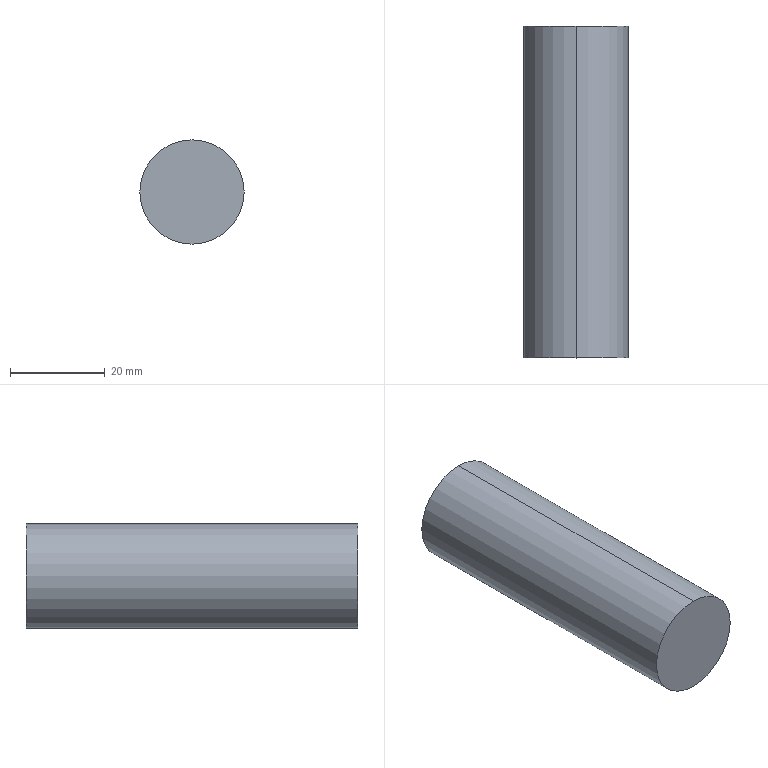Part | SolidWorks | features Extrusion 1, HoleWzd 1 | 1 solid | 8 faces | box 22 x 70 x 22 mm | volume 25142 mm3 | cylinder 4 | cone 2 | plane 2 | commonest cylinder face diameters 8.5 x2 22 x2
STEP:
#1=CARTESIAN_POINT('',(0.,45.,-4.25));
#2=VERTEX_POINT('',#1);
#3=CARTESIAN_POINT('',(0.,45.,4.25));
#4=VERTEX_POINT('',#3);
#5=CARTESIAN_POINT('',(0.,45.,0.));
#6=DIRECTION('',(0.,1.,0.));
#7=DIRECTION('',(0.,0.,1.));
#8=AXIS2_PLACEMENT_3D('',#5,#6,#7);
#9=CIRCLE('',#8,4.25);
#10=EDGE_CURVE('',#2,#4,#9,.T.);
#11=ORIENTED_EDGE('',*,*,#10,.F.);
#12=CARTESIAN_POINT('',(0.,70.,-4.25));
#13=VERTEX_POINT('',#12);
#14=CARTESIAN_POINT('',(0.,70.,-4.25));
#15=DIRECTION('',(0.,1.,0.));
#16=VECTOR('',#15,1000.);
#17=LINE('',#14,#16);
#18=EDGE_CURVE('',#2,#13,#17,.T.);
#19=ORIENTED_EDGE('',*,*,#18,.T.);
#20=CARTESIAN_POINT('',(0.,70.,4.25));
#21=VERTEX_POINT('',#20);
#22=CARTESIAN_POINT('',(0.,70.,0.));
#23=DIRECTION('',(0.,1.,0.));
#24=DIRECTION('',(0.,0.,1.));
#25=AXIS2_PLACEMENT_3D('',#22,#23,#24);
#26=CIRCLE('',#25,4.25);
#27=EDGE_CURVE('',#13,#21,#26,.T.);
#28=ORIENTED_EDGE('',*,*,#27,.T.);
#29=CARTESIAN_POINT('',(0.,70.,4.25));
#30=DIRECTION('',(0.,1.,0.));
#31=VECTOR('',#30,1000.);
#32=LINE('',#29,#31);
#33=EDGE_CURVE('',#4,#21,#32,.T.);
#34=ORIENTED_EDGE('',*,*,#33,.F.);
#35=EDGE_LOOP('',(#11,#19,#28,#34));
#36=FACE_OUTER_BOUND('',#35,.T.);
#37=CARTESIAN_POINT('',(0.,70.,0.));
#38=DIRECTION('',(0.,1.,0.));
#39=DIRECTION('',(0.,0.,1.));
#40=AXIS2_PLACEMENT_3D('',#37,#38,#39);
#41=CYLINDRICAL_SURFACE('',#40,4.25);
#42=ADVANCED_FACE('',(#36),#41,.F.);
#43=CARTESIAN_POINT('',(0.,42.446,0.));
#44=VERTEX_POINT('',#43);
#45=CARTESIAN_POINT('',(0.,45.,4.25));
#46=DIRECTION('',(0.,0.515,0.8572));
#47=VECTOR('',#46,1000.);
#48=LINE('',#45,#47);
#49=EDGE_CURVE('',#44,#4,#48,.T.);
#50=ORIENTED_EDGE('',*,*,#49,.F.);
#51=CARTESIAN_POINT('',(0.,45.,-4.25));
#52=DIRECTION('',(0.,0.515,-0.8572));
#53=VECTOR('',#52,1000.);
#54=LINE('',#51,#53);
#55=EDGE_CURVE('',#44,#2,#54,.T.);
#56=ORIENTED_EDGE('',*,*,#55,.T.);
#57=ORIENTED_EDGE('',*,*,#10,.T.);
#58=EDGE_LOOP('',(#50,#56,#57));
#59=FACE_OUTER_BOUND('',#58,.T.);
#60=CARTESIAN_POINT('',(0.,45.,0.));
#61=DIRECTION('',(0.,1.,0.));
#62=DIRECTION('',(0.,0.,1.));
#63=AXIS2_PLACEMENT_3D('',#60,#61,#62);
#64=CONICAL_SURFACE('',#63,4.25,1.03);
#65=ADVANCED_FACE('',(#59),#64,.F.);
#66=CARTESIAN_POINT('',(0.,70.,11.));
#67=VERTEX_POINT('',#66);
#68=CARTESIAN_POINT('',(0.,70.,-11.));
#69=VERTEX_POINT('',#68);
#70=CARTESIAN_POINT('',(0.,70.,0.));
#71=DIRECTION('',(0.,1.,0.));
#72=DIRECTION('',(0.,0.,1.));
#73=AXIS2_PLACEMENT_3D('',#70,#71,#72);
#74=CIRCLE('',#73,11.);
#75=EDGE_CURVE('',#67,#69,#74,.T.);
#76=ORIENTED_EDGE('',*,*,#75,.F.);
#77=CARTESIAN_POINT('',(0.,0.,11.));
#78=VERTEX_POINT('',#77);
#79=CARTESIAN_POINT('',(0.,70.,11.));
#80=DIRECTION('',(0.,-1.,0.));
#81=VECTOR('',#80,1000.);
#82=LINE('',#79,#81);
#83=EDGE_CURVE('',#67,#78,#82,.T.);
#84=ORIENTED_EDGE('',*,*,#83,.T.);
#85=CARTESIAN_POINT('',(0.,0.,-11.));
#86=VERTEX_POINT('',#85);
#87=CARTESIAN_POINT('',(0.,0.,0.));
#88=DIRECTION('',(0.,1.,0.));
#89=DIRECTION('',(0.,0.,1.));
#90=AXIS2_PLACEMENT_3D('',#87,#88,#89);
#91=CIRCLE('',#90,11.);
#92=EDGE_CURVE('',#78,#86,#91,.T.);
#93=ORIENTED_EDGE('',*,*,#92,.T.);
#94=CARTESIAN_POINT('',(0.,70.,-11.));
#95=DIRECTION('',(0.,-1.,0.));
#96=VECTOR('',#95,1000.);
#97=LINE('',#94,#96);
#98=EDGE_CURVE('',#69,#86,#97,.T.);
#99=ORIENTED_EDGE('',*,*,#98,.F.);
#100=EDGE_LOOP('',(#76,#84,#93,#99));
#101=FACE_OUTER_BOUND('',#100,.T.);
#102=CARTESIAN_POINT('',(0.,70.,0.));
#103=DIRECTION('',(0.,-1.,0.));
#104=DIRECTION('',(0.,0.,-1.));
#105=AXIS2_PLACEMENT_3D('',#102,#103,#104);
#106=CYLINDRICAL_SURFACE('',#105,11.);
#107=ADVANCED_FACE('',(#101),#106,.T.);
#108=ORIENTED_EDGE('',*,*,#83,.F.);
#109=CARTESIAN_POINT('',(0.,70.,0.));
#110=DIRECTION('',(0.,1.,0.));
#111=DIRECTION('',(0.,0.,1.));
#112=AXIS2_PLACEMENT_3D('',#109,#110,#111);
#113=CIRCLE('',#112,11.);
#114=EDGE_CURVE('',#69,#67,#113,.T.);
#115=ORIENTED_EDGE('',*,*,#114,.F.);
#116=ORIENTED_EDGE('',*,*,#98,.T.);
#117=CARTESIAN_POINT('',(0.,0.,0.));
#118=DIRECTION('',(0.,1.,0.));
#119=DIRECTION('',(0.,0.,1.));
#120=AXIS2_PLACEMENT_3D('',#117,#118,#119);
#121=CIRCLE('',#120,11.);
#122=EDGE_CURVE('',#86,#78,#121,.T.);
#123=ORIENTED_EDGE('',*,*,#122,.T.);
#124=EDGE_LOOP('',(#108,#115,#116,#123));
#125=FACE_OUTER_BOUND('',#124,.T.);
#126=CARTESIAN_POINT('',(0.,70.,0.));
#127=DIRECTION('',(0.,-1.,0.));
#128=DIRECTION('',(0.,0.,-1.));
#129=AXIS2_PLACEMENT_3D('',#126,#127,#128);
#130=CYLINDRICAL_SURFACE('',#129,11.);
#131=ADVANCED_FACE('',(#125),#130,.T.);
#132=CARTESIAN_POINT('',(0.,70.,0.));
#133=DIRECTION('',(0.,1.,0.));
#134=DIRECTION('',(0.,0.,1.));
#135=AXIS2_PLACEMENT_3D('',#132,#133,#134);
#136=CIRCLE('',#135,4.25);
#137=EDGE_CURVE('',#21,#13,#136,.T.);
#138=ORIENTED_EDGE('',*,*,#137,.F.);
#139=ORIENTED_EDGE('',*,*,#27,.F.);
#140=EDGE_LOOP('',(#138,#139));
#141=FACE_BOUND('',#140,.T.);
#142=ORIENTED_EDGE('',*,*,#114,.T.);
#143=ORIENTED_EDGE('',*,*,#75,.T.);
#144=EDGE_LOOP('',(#142,#143));
#145=FACE_OUTER_BOUND('',#144,.T.);
#146=CARTESIAN_POINT('',(0.,70.,0.));
#147=DIRECTION('',(0.,1.,0.));
#148=DIRECTION('',(0.,0.,1.));
#149=AXIS2_PLACEMENT_3D('',#146,#147,#148);
#150=PLANE('',#149);
#151=ADVANCED_FACE('',(#141,#145),#150,.T.);
#152=ORIENTED_EDGE('',*,*,#122,.F.);
#153=ORIENTED_EDGE('',*,*,#92,.F.);
#154=EDGE_LOOP('',(#152,#153));
#155=FACE_OUTER_BOUND('',#154,.T.);
#156=CARTESIAN_POINT('',(0.,0.,0.));
#157=DIRECTION('',(0.,1.,0.));
#158=DIRECTION('',(0.,0.,1.));
#159=AXIS2_PLACEMENT_3D('',#156,#157,#158);
#160=PLANE('',#159);
#161=ADVANCED_FACE('',(#155),#160,.F.);
#162=ORIENTED_EDGE('',*,*,#55,.F.);
#163=ORIENTED_EDGE('',*,*,#49,.T.);
#164=CARTESIAN_POINT('',(0.,45.,0.));
#165=DIRECTION('',(0.,1.,0.));
#166=DIRECTION('',(0.,0.,1.));
#167=AXIS2_PLACEMENT_3D('',#164,#165,#166);
#168=CIRCLE('',#167,4.25);
#169=EDGE_CURVE('',#4,#2,#168,.T.);
#170=ORIENTED_EDGE('',*,*,#169,.T.);
#171=EDGE_LOOP('',(#162,#163,#170));
#172=FACE_OUTER_BOUND('',#171,.T.);
#173=CARTESIAN_POINT('',(0.,45.,0.));
#174=DIRECTION('',(0.,1.,0.));
#175=DIRECTION('',(0.,0.,1.));
#176=AXIS2_PLACEMENT_3D('',#173,#174,#175);
#177=CONICAL_SURFACE('',#176,4.25,1.03);
#178=ADVANCED_FACE('',(#172),#177,.F.);
#179=ORIENTED_EDGE('',*,*,#18,.F.);
#180=ORIENTED_EDGE('',*,*,#169,.F.);
#181=ORIENTED_EDGE('',*,*,#33,.T.);
#182=ORIENTED_EDGE('',*,*,#137,.T.);
#183=EDGE_LOOP('',(#179,#180,#181,#182));
#184=FACE_OUTER_BOUND('',#183,.T.);
#185=CARTESIAN_POINT('',(0.,70.,0.));
#186=DIRECTION('',(0.,1.,0.));
#187=DIRECTION('',(0.,0.,1.));
#188=AXIS2_PLACEMENT_3D('',#185,#186,#187);
#189=CYLINDRICAL_SURFACE('',#188,4.25);
#190=ADVANCED_FACE('',(#184),#189,.F.);
#191=CLOSED_SHELL('',(#42,#65,#107,#131,#151,#161,#178,#190));
#192=MANIFOLD_SOLID_BREP('',#191);
#193=CARTESIAN_POINT('',(0.,0.,0.));
#194=DIRECTION('',(0.,0.,1.));
#195=DIRECTION('',(1.,0.,0.));
#196=AXIS2_PLACEMENT_3D('',#193,#194,#195);
#197=(LENGTH_UNIT()NAMED_UNIT(*)SI_UNIT(.MILLI.,.METRE.));
#198=UNCERTAINTY_MEASURE_WITH_UNIT(LENGTH_MEASURE(0.00001),#197,'','');
#199=(NAMED_UNIT(*)PLANE_ANGLE_UNIT()SI_UNIT($,.RADIAN.));
#200=(NAMED_UNIT(*)SI_UNIT($,.STERADIAN.)SOLID_ANGLE_UNIT());
#201=(GEOMETRIC_REPRESENTATION_CONTEXT(3)GLOBAL_UNCERTAINTY_ASSIGNED_CONTEXT((#198))GLOBAL_UNIT_ASSIGNED_CONTEXT((#197,#199,#200))REPRESENTATION_CONTEXT('',''));
#202=ADVANCED_BREP_SHAPE_REPRESENTATION('',(#192,#196),#201);